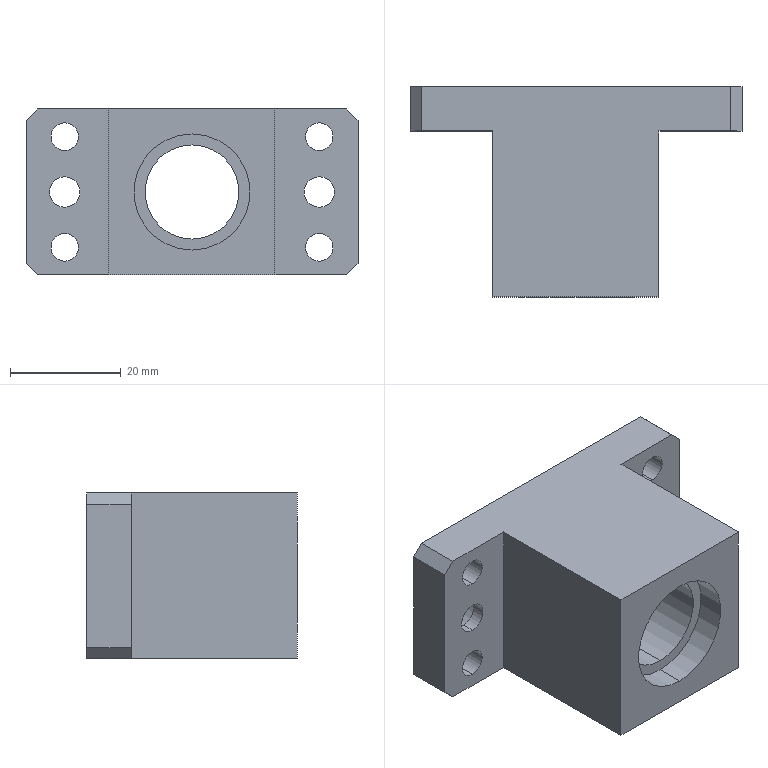Part | NX | features BREP 1 | 1 solid | 40 faces | box 60 x 38 x 30 mm | volume 29884 mm3 | cylinder 22 | plane 18 | commonest cylinder face diameters 5 x8 5.5 x4 10 x4 21 x4 17 x2
STEP:
#1=CARTESIAN_POINT('',(-23.,-8.,-12.5));
#2=VERTEX_POINT('',#1);
#3=CARTESIAN_POINT('',(-23.,-8.,-7.5));
#4=VERTEX_POINT('',#3);
#5=CARTESIAN_POINT('',(-23.,-8.,-10.));
#6=DIRECTION('',(0.,1.,0.));
#7=DIRECTION('',(-1.,0.,0.));
#8=AXIS2_PLACEMENT_3D('',#5,#6,#7);
#9=CIRCLE('',#8,2.5);
#10=EDGE_CURVE('',#2,#4,#9,.T.);
#11=ORIENTED_EDGE('',*,*,#10,.F.);
#12=CARTESIAN_POINT('',(-23.,0.,-12.5));
#13=VERTEX_POINT('',#12);
#14=CARTESIAN_POINT('',(-23.,0.,-12.5));
#15=DIRECTION('',(0.,1.,0.));
#16=VECTOR('',#15,1000.);
#17=LINE('',#14,#16);
#18=EDGE_CURVE('',#2,#13,#17,.T.);
#19=ORIENTED_EDGE('',*,*,#18,.T.);
#20=CARTESIAN_POINT('',(-23.,0.,-7.5));
#21=VERTEX_POINT('',#20);
#22=CARTESIAN_POINT('',(-23.,0.,-10.));
#23=DIRECTION('',(0.,1.,0.));
#24=DIRECTION('',(0.,0.,1.));
#25=AXIS2_PLACEMENT_3D('',#22,#23,#24);
#26=CIRCLE('',#25,2.5);
#27=EDGE_CURVE('',#13,#21,#26,.T.);
#28=ORIENTED_EDGE('',*,*,#27,.T.);
#29=CARTESIAN_POINT('',(-23.,0.,-7.5));
#30=DIRECTION('',(0.,1.,0.));
#31=VECTOR('',#30,1000.);
#32=LINE('',#29,#31);
#33=EDGE_CURVE('',#4,#21,#32,.T.);
#34=ORIENTED_EDGE('',*,*,#33,.F.);
#35=EDGE_LOOP('',(#11,#19,#28,#34));
#36=FACE_BOUND('',#35,.T.);
#37=CARTESIAN_POINT('',(-23.,0.,-10.));
#38=DIRECTION('',(0.,1.,0.));
#39=DIRECTION('',(0.,0.,-1.));
#40=AXIS2_PLACEMENT_3D('',#37,#38,#39);
#41=CYLINDRICAL_SURFACE('',#40,2.5);
#42=ADVANCED_FACE('',(#36),#41,.F.);
#43=CARTESIAN_POINT('',(23.,-8.,-12.5));
#44=VERTEX_POINT('',#43);
#45=CARTESIAN_POINT('',(23.,-8.,-7.5));
#46=VERTEX_POINT('',#45);
#47=CARTESIAN_POINT('',(23.,-8.,-10.));
#48=DIRECTION('',(0.,1.,0.));
#49=DIRECTION('',(-1.,0.,0.));
#50=AXIS2_PLACEMENT_3D('',#47,#48,#49);
#51=CIRCLE('',#50,2.5);
#52=EDGE_CURVE('',#44,#46,#51,.T.);
#53=ORIENTED_EDGE('',*,*,#52,.F.);
#54=CARTESIAN_POINT('',(23.,0.,-12.5));
#55=VERTEX_POINT('',#54);
#56=CARTESIAN_POINT('',(23.,0.,-12.5));
#57=DIRECTION('',(0.,1.,0.));
#58=VECTOR('',#57,1000.);
#59=LINE('',#56,#58);
#60=EDGE_CURVE('',#44,#55,#59,.T.);
#61=ORIENTED_EDGE('',*,*,#60,.T.);
#62=CARTESIAN_POINT('',(23.,0.,-7.5));
#63=VERTEX_POINT('',#62);
#64=CARTESIAN_POINT('',(23.,0.,-10.));
#65=DIRECTION('',(0.,1.,0.));
#66=DIRECTION('',(0.,0.,1.));
#67=AXIS2_PLACEMENT_3D('',#64,#65,#66);
#68=CIRCLE('',#67,2.5);
#69=EDGE_CURVE('',#55,#63,#68,.T.);
#70=ORIENTED_EDGE('',*,*,#69,.T.);
#71=CARTESIAN_POINT('',(23.,0.,-7.5));
#72=DIRECTION('',(0.,1.,0.));
#73=VECTOR('',#72,1000.);
#74=LINE('',#71,#73);
#75=EDGE_CURVE('',#46,#63,#74,.T.);
#76=ORIENTED_EDGE('',*,*,#75,.F.);
#77=EDGE_LOOP('',(#53,#61,#70,#76));
#78=FACE_BOUND('',#77,.T.);
#79=CARTESIAN_POINT('',(23.,0.,-10.));
#80=DIRECTION('',(0.,1.,0.));
#81=DIRECTION('',(0.,0.,-1.));
#82=AXIS2_PLACEMENT_3D('',#79,#80,#81);
#83=CYLINDRICAL_SURFACE('',#82,2.5);
#84=ADVANCED_FACE('',(#78),#83,.F.);
#85=CARTESIAN_POINT('',(23.,-8.,7.5));
#86=VERTEX_POINT('',#85);
#87=CARTESIAN_POINT('',(23.,-8.,12.5));
#88=VERTEX_POINT('',#87);
#89=CARTESIAN_POINT('',(23.,-8.,10.));
#90=DIRECTION('',(0.,1.,0.));
#91=DIRECTION('',(-1.,0.,0.));
#92=AXIS2_PLACEMENT_3D('',#89,#90,#91);
#93=CIRCLE('',#92,2.5);
#94=EDGE_CURVE('',#86,#88,#93,.T.);
#95=ORIENTED_EDGE('',*,*,#94,.F.);
#96=CARTESIAN_POINT('',(23.,0.,7.5));
#97=VERTEX_POINT('',#96);
#98=CARTESIAN_POINT('',(23.,0.,7.5));
#99=DIRECTION('',(0.,1.,0.));
#100=VECTOR('',#99,1000.);
#101=LINE('',#98,#100);
#102=EDGE_CURVE('',#86,#97,#101,.T.);
#103=ORIENTED_EDGE('',*,*,#102,.T.);
#104=CARTESIAN_POINT('',(23.,0.,12.5));
#105=VERTEX_POINT('',#104);
#106=CARTESIAN_POINT('',(23.,0.,10.));
#107=DIRECTION('',(0.,1.,0.));
#108=DIRECTION('',(0.,0.,1.));
#109=AXIS2_PLACEMENT_3D('',#106,#107,#108);
#110=CIRCLE('',#109,2.5);
#111=EDGE_CURVE('',#97,#105,#110,.T.);
#112=ORIENTED_EDGE('',*,*,#111,.T.);
#113=CARTESIAN_POINT('',(23.,0.,12.5));
#114=DIRECTION('',(0.,1.,0.));
#115=VECTOR('',#114,1000.);
#116=LINE('',#113,#115);
#117=EDGE_CURVE('',#88,#105,#116,.T.);
#118=ORIENTED_EDGE('',*,*,#117,.F.);
#119=EDGE_LOOP('',(#95,#103,#112,#118));
#120=FACE_BOUND('',#119,.T.);
#121=CARTESIAN_POINT('',(23.,0.,10.));
#122=DIRECTION('',(0.,1.,0.));
#123=DIRECTION('',(0.,0.,-1.));
#124=AXIS2_PLACEMENT_3D('',#121,#122,#123);
#125=CYLINDRICAL_SURFACE('',#124,2.5);
#126=ADVANCED_FACE('',(#120),#125,.F.);
#127=CARTESIAN_POINT('',(-23.,-8.,7.5));
#128=VERTEX_POINT('',#127);
#129=CARTESIAN_POINT('',(-23.,-8.,12.5));
#130=VERTEX_POINT('',#129);
#131=CARTESIAN_POINT('',(-23.,-8.,10.));
#132=DIRECTION('',(0.,1.,0.));
#133=DIRECTION('',(-1.,0.,0.));
#134=AXIS2_PLACEMENT_3D('',#131,#132,#133);
#135=CIRCLE('',#134,2.5);
#136=EDGE_CURVE('',#128,#130,#135,.T.);
#137=ORIENTED_EDGE('',*,*,#136,.F.);
#138=CARTESIAN_POINT('',(-23.,0.,7.5));
#139=VERTEX_POINT('',#138);
#140=CARTESIAN_POINT('',(-23.,0.,7.5));
#141=DIRECTION('',(0.,1.,0.));
#142=VECTOR('',#141,1000.);
#143=LINE('',#140,#142);
#144=EDGE_CURVE('',#128,#139,#143,.T.);
#145=ORIENTED_EDGE('',*,*,#144,.T.);
#146=CARTESIAN_POINT('',(-23.,0.,12.5));
#147=VERTEX_POINT('',#146);
#148=CARTESIAN_POINT('',(-23.,0.,10.));
#149=DIRECTION('',(0.,1.,0.));
#150=DIRECTION('',(0.,0.,1.));
#151=AXIS2_PLACEMENT_3D('',#148,#149,#150);
#152=CIRCLE('',#151,2.5);
#153=EDGE_CURVE('',#139,#147,#152,.T.);
#154=ORIENTED_EDGE('',*,*,#153,.T.);
#155=CARTESIAN_POINT('',(-23.,0.,12.5));
#156=DIRECTION('',(0.,1.,0.));
#157=VECTOR('',#156,1000.);
#158=LINE('',#155,#157);
#159=EDGE_CURVE('',#130,#147,#158,.T.);
#160=ORIENTED_EDGE('',*,*,#159,.F.);
#161=EDGE_LOOP('',(#137,#145,#154,#160));
#162=FACE_BOUND('',#161,.T.);
#163=CARTESIAN_POINT('',(-23.,0.,10.));
#164=DIRECTION('',(0.,1.,0.));
#165=DIRECTION('',(0.,0.,-1.));
#166=AXIS2_PLACEMENT_3D('',#163,#164,#165);
#167=CYLINDRICAL_SURFACE('',#166,2.5);
#168=ADVANCED_FACE('',(#162),#167,.F.);
#169=CARTESIAN_POINT('',(0.,-33.,8.5));
#170=VERTEX_POINT('',#169);
#171=CARTESIAN_POINT('',(0.,-33.,-8.5));
#172=VERTEX_POINT('',#171);
#173=CARTESIAN_POINT('',(0.,-33.,0.));
#174=DIRECTION('',(0.,-1.,0.));
#175=DIRECTION('',(0.,0.,-1.));
#176=AXIS2_PLACEMENT_3D('',#173,#174,#175);
#177=CIRCLE('',#176,8.5);
#178=EDGE_CURVE('',#170,#172,#177,.T.);
#179=ORIENTED_EDGE('',*,*,#178,.T.);
#180=CARTESIAN_POINT('',(0.,-5.,-8.5));
#181=VERTEX_POINT('',#180);
#182=CARTESIAN_POINT('',(0.,-38.,-8.5));
#183=DIRECTION('',(0.,1.,0.));
#184=VECTOR('',#183,1000.);
#185=LINE('',#182,#184);
#186=EDGE_CURVE('',#172,#181,#185,.T.);
#187=ORIENTED_EDGE('',*,*,#186,.T.);
#188=CARTESIAN_POINT('',(0.,-5.,8.5));
#189=VERTEX_POINT('',#188);
#190=CARTESIAN_POINT('',(0.,-5.,0.));
#191=DIRECTION('',(0.,1.,0.));
#192=DIRECTION('',(0.,0.,1.));
#193=AXIS2_PLACEMENT_3D('',#190,#191,#192);
#194=CIRCLE('',#193,8.5);
#195=EDGE_CURVE('',#181,#189,#194,.T.);
#196=ORIENTED_EDGE('',*,*,#195,.T.);
#197=CARTESIAN_POINT('',(0.,-38.,8.5));
#198=DIRECTION('',(0.,1.,0.));
#199=VECTOR('',#198,1000.);
#200=LINE('',#197,#199);
#201=EDGE_CURVE('',#170,#189,#200,.T.);
#202=ORIENTED_EDGE('',*,*,#201,.F.);
#203=EDGE_LOOP('',(#179,#187,#196,#202));
#204=FACE_BOUND('',#203,.T.);
#205=CARTESIAN_POINT('',(0.,-38.,0.));
#206=DIRECTION('',(0.,1.,0.));
#207=DIRECTION('',(0.,0.,-1.));
#208=AXIS2_PLACEMENT_3D('',#205,#206,#207);
#209=CYLINDRICAL_SURFACE('',#208,8.5);
#210=ADVANCED_FACE('',(#204),#209,.F.);
#211=CARTESIAN_POINT('',(0.,-33.,10.5));
#212=VERTEX_POINT('',#211);
#213=CARTESIAN_POINT('',(0.,-33.,-10.5));
#214=VERTEX_POINT('',#213);
#215=CARTESIAN_POINT('',(0.,-33.,0.));
#216=DIRECTION('',(0.,-1.,0.));
#217=DIRECTION('',(0.,0.,-1.));
#218=AXIS2_PLACEMENT_3D('',#215,#216,#217);
#219=CIRCLE('',#218,10.5);
#220=EDGE_CURVE('',#212,#214,#219,.T.);
#221=ORIENTED_EDGE('',*,*,#220,.F.);
#222=CARTESIAN_POINT('',(0.,-38.,10.5));
#223=VERTEX_POINT('',#222);
#224=CARTESIAN_POINT('',(0.,-33.,10.5));
#225=DIRECTION('',(0.,-1.,0.));
#226=VECTOR('',#225,1000.);
#227=LINE('',#224,#226);
#228=EDGE_CURVE('',#223,#212,#227,.F.);
#229=ORIENTED_EDGE('',*,*,#228,.F.);
#230=CARTESIAN_POINT('',(0.,-38.,-10.5));
#231=VERTEX_POINT('',#230);
#232=CARTESIAN_POINT('',(0.,-38.,0.));
#233=DIRECTION('',(0.,-1.,0.));
#234=DIRECTION('',(0.,0.,-1.));
#235=AXIS2_PLACEMENT_3D('',#232,#233,#234);
#236=CIRCLE('',#235,10.5);
#237=EDGE_CURVE('',#223,#231,#236,.T.);
#238=ORIENTED_EDGE('',*,*,#237,.T.);
#239=CARTESIAN_POINT('',(0.,-33.,-10.5));
#240=DIRECTION('',(0.,-1.,0.));
#241=VECTOR('',#240,1000.);
#242=LINE('',#239,#241);
#243=EDGE_CURVE('',#231,#214,#242,.F.);
#244=ORIENTED_EDGE('',*,*,#243,.T.);
#245=EDGE_LOOP('',(#221,#229,#238,#244));
#246=FACE_BOUND('',#245,.T.);
#247=CARTESIAN_POINT('',(0.,-33.,0.));
#248=DIRECTION('',(0.,-1.,0.));
#249=DIRECTION('',(0.,0.,1.));
#250=AXIS2_PLACEMENT_3D('',#247,#248,#249);
#251=CYLINDRICAL_SURFACE('',#250,10.5);
#252=ADVANCED_FACE('',(#246),#251,.F.);
#253=CARTESIAN_POINT('',(0.,-5.,-10.5));
#254=VERTEX_POINT('',#253);
#255=CARTESIAN_POINT('',(0.,-5.,10.5));
#256=VERTEX_POINT('',#255);
#257=CARTESIAN_POINT('',(0.,-5.,0.));
#258=DIRECTION('',(0.,1.,0.));
#259=DIRECTION('',(0.,0.,1.));
#260=AXIS2_PLACEMENT_3D('',#257,#258,#259);
#261=CIRCLE('',#260,10.5);
#262=EDGE_CURVE('',#254,#256,#261,.T.);
#263=ORIENTED_EDGE('',*,*,#262,.F.);
#264=CARTESIAN_POINT('',(0.,0.,-10.5));
#265=VERTEX_POINT('',#264);
#266=CARTESIAN_POINT('',(0.,-5.,-10.5));
#267=DIRECTION('',(0.,1.,0.));
#268=VECTOR('',#267,1000.);
#269=LINE('',#266,#268);
#270=EDGE_CURVE('',#254,#265,#269,.T.);
#271=ORIENTED_EDGE('',*,*,#270,.T.);
#272=CARTESIAN_POINT('',(0.,0.,10.5));
#273=VERTEX_POINT('',#272);
#274=CARTESIAN_POINT('',(0.,0.,0.));
#275=DIRECTION('',(0.,1.,0.));
#276=DIRECTION('',(0.,0.,1.));
#277=AXIS2_PLACEMENT_3D('',#274,#275,#276);
#278=CIRCLE('',#277,10.5);
#279=EDGE_CURVE('',#265,#273,#278,.T.);
#280=ORIENTED_EDGE('',*,*,#279,.T.);
#281=CARTESIAN_POINT('',(0.,-5.,10.5));
#282=DIRECTION('',(0.,1.,0.));
#283=VECTOR('',#282,1000.);
#284=LINE('',#281,#283);
#285=EDGE_CURVE('',#256,#273,#284,.T.);
#286=ORIENTED_EDGE('',*,*,#285,.F.);
#287=EDGE_LOOP('',(#263,#271,#280,#286));
#288=FACE_BOUND('',#287,.T.);
#289=CARTESIAN_POINT('',(0.,-5.,0.));
#290=DIRECTION('',(0.,1.,0.));
#291=DIRECTION('',(0.,0.,-1.));
#292=AXIS2_PLACEMENT_3D('',#289,#290,#291);
#293=CYLINDRICAL_SURFACE('',#292,10.5);
#294=ADVANCED_FACE('',(#288),#293,.F.);
#295=CARTESIAN_POINT('',(23.,-5.7,-5.));
#296=VERTEX_POINT('',#295);
#297=CARTESIAN_POINT('',(23.,-5.7,5.));
#298=VERTEX_POINT('',#297);
#299=CARTESIAN_POINT('',(23.,-5.7,0.));
#300=DIRECTION('',(0.,1.,0.));
#301=DIRECTION('',(0.,0.,1.));
#302=AXIS2_PLACEMENT_3D('',#299,#300,#301);
#303=CIRCLE('',#302,5.);
#304=EDGE_CURVE('',#296,#298,#303,.T.);
#305=ORIENTED_EDGE('',*,*,#304,.F.);
#306=CARTESIAN_POINT('',(23.,0.,-5.));
#307=VERTEX_POINT('',#306);
#308=CARTESIAN_POINT('',(23.,0.,-5.));
#309=DIRECTION('',(0.,1.,0.));
#310=VECTOR('',#309,1000.);
#311=LINE('',#308,#310);
#312=EDGE_CURVE('',#296,#307,#311,.T.);
#313=ORIENTED_EDGE('',*,*,#312,.T.);
#314=CARTESIAN_POINT('',(23.,0.,5.));
#315=VERTEX_POINT('',#314);
#316=CARTESIAN_POINT('',(23.,0.,0.));
#317=DIRECTION('',(0.,1.,0.));
#318=DIRECTION('',(0.,0.,1.));
#319=AXIS2_PLACEMENT_3D('',#316,#317,#318);
#320=CIRCLE('',#319,5.);
#321=EDGE_CURVE('',#307,#315,#320,.T.);
#322=ORIENTED_EDGE('',*,*,#321,.T.);
#323=CARTESIAN_POINT('',(23.,0.,5.));
#324=DIRECTION('',(0.,1.,0.));
#325=VECTOR('',#324,1000.);
#326=LINE('',#323,#325);
#327=EDGE_CURVE('',#298,#315,#326,.T.);
#328=ORIENTED_EDGE('',*,*,#327,.F.);
#329=EDGE_LOOP('',(#305,#313,#322,#328));
#330=FACE_BOUND('',#329,.T.);
#331=CARTESIAN_POINT('',(23.,0.,0.));
#332=DIRECTION('',(0.,1.,0.));
#333=DIRECTION('',(0.,0.,-1.));
#334=AXIS2_PLACEMENT_3D('',#331,#332,#333);
#335=CYLINDRICAL_SURFACE('',#334,5.);
#336=ADVANCED_FACE('',(#330),#335,.F.);
#337=CARTESIAN_POINT('',(23.,-8.,-2.75));
#338=VERTEX_POINT('',#337);
#339=CARTESIAN_POINT('',(23.,-8.,2.75));
#340=VERTEX_POINT('',#339);
#341=CARTESIAN_POINT('',(23.,-8.,0.));
#342=DIRECTION('',(0.,1.,0.));
#343=DIRECTION('',(-1.,0.,0.));
#344=AXIS2_PLACEMENT_3D('',#341,#342,#343);
#345=CIRCLE('',#344,2.75);
#346=EDGE_CURVE('',#338,#340,#345,.T.);
#347=ORIENTED_EDGE('',*,*,#346,.F.);
#348=CARTESIAN_POINT('',(23.,-5.7,-2.75));
#349=VERTEX_POINT('',#348);
#350=CARTESIAN_POINT('',(23.,0.,-2.75));
#351=DIRECTION('',(0.,1.,0.));
#352=VECTOR('',#351,1000.);
#353=LINE('',#350,#352);
#354=EDGE_CURVE('',#338,#349,#353,.T.);
#355=ORIENTED_EDGE('',*,*,#354,.T.);
#356=CARTESIAN_POINT('',(23.,-5.7,2.75));
#357=VERTEX_POINT('',#356);
#358=CARTESIAN_POINT('',(23.,-5.7,0.));
#359=DIRECTION('',(0.,1.,0.));
#360=DIRECTION('',(0.,0.,1.));
#361=AXIS2_PLACEMENT_3D('',#358,#359,#360);
#362=CIRCLE('',#361,2.75);
#363=EDGE_CURVE('',#349,#357,#362,.T.);
#364=ORIENTED_EDGE('',*,*,#363,.T.);
#365=CARTESIAN_POINT('',(23.,0.,2.75));
#366=DIRECTION('',(0.,1.,0.));
#367=VECTOR('',#366,1000.);
#368=LINE('',#365,#367);
#369=EDGE_CURVE('',#340,#357,#368,.T.);
#370=ORIENTED_EDGE('',*,*,#369,.F.);
#371=EDGE_LOOP('',(#347,#355,#364,#370));
#372=FACE_BOUND('',#371,.T.);
#373=CARTESIAN_POINT('',(23.,0.,0.));
#374=DIRECTION('',(0.,1.,0.));
#375=DIRECTION('',(0.,0.,-1.));
#376=AXIS2_PLACEMENT_3D('',#373,#374,#375);
#377=CYLINDRICAL_SURFACE('',#376,2.75);
#378=ADVANCED_FACE('',(#372),#377,.F.);
#379=CARTESIAN_POINT('',(-23.,-5.7,-5.));
#380=VERTEX_POINT('',#379);
#381=CARTESIAN_POINT('',(-23.,-5.7,5.));
#382=VERTEX_POINT('',#381);
#383=CARTESIAN_POINT('',(-23.,-5.7,0.));
#384=DIRECTION('',(0.,1.,0.));
#385=DIRECTION('',(0.,0.,1.));
#386=AXIS2_PLACEMENT_3D('',#383,#384,#385);
#387=CIRCLE('',#386,5.);
#388=EDGE_CURVE('',#380,#382,#387,.T.);
#389=ORIENTED_EDGE('',*,*,#388,.F.);
#390=CARTESIAN_POINT('',(-23.,0.,-5.));
#391=VERTEX_POINT('',#390);
#392=CARTESIAN_POINT('',(-23.,0.,-5.));
#393=DIRECTION('',(0.,1.,0.));
#394=VECTOR('',#393,1000.);
#395=LINE('',#392,#394);
#396=EDGE_CURVE('',#380,#391,#395,.T.);
#397=ORIENTED_EDGE('',*,*,#396,.T.);
#398=CARTESIAN_POINT('',(-23.,0.,5.));
#399=VERTEX_POINT('',#398);
#400=CARTESIAN_POINT('',(-23.,0.,0.));
#401=DIRECTION('',(0.,1.,0.));
#402=DIRECTION('',(0.,0.,1.));
#403=AXIS2_PLACEMENT_3D('',#400,#401,#402);
#404=CIRCLE('',#403,5.);
#405=EDGE_CURVE('',#391,#399,#404,.T.);
#406=ORIENTED_EDGE('',*,*,#405,.T.);
#407=CARTESIAN_POINT('',(-23.,0.,5.));
#408=DIRECTION('',(0.,1.,0.));
#409=VECTOR('',#408,1000.);
#410=LINE('',#407,#409);
#411=EDGE_CURVE('',#382,#399,#410,.T.);
#412=ORIENTED_EDGE('',*,*,#411,.F.);
#413=EDGE_LOOP('',(#389,#397,#406,#412));
#414=FACE_BOUND('',#413,.T.);
#415=CARTESIAN_POINT('',(-23.,0.,0.));
#416=DIRECTION('',(0.,1.,0.));
#417=DIRECTION('',(0.,0.,-1.));
#418=AXIS2_PLACEMENT_3D('',#415,#416,#417);
#419=CYLINDRICAL_SURFACE('',#418,5.);
#420=ADVANCED_FACE('',(#414),#419,.F.);
#421=CARTESIAN_POINT('',(-23.,-8.,-2.75));
#422=VERTEX_POINT('',#421);
#423=CARTESIAN_POINT('',(-23.,-8.,2.75));
#424=VERTEX_POINT('',#423);
#425=CARTESIAN_POINT('',(-23.,-8.,0.));
#426=DIRECTION('',(0.,1.,0.));
#427=DIRECTION('',(-1.,0.,0.));
#428=AXIS2_PLACEMENT_3D('',#425,#426,#427);
#429=CIRCLE('',#428,2.75);
#430=EDGE_CURVE('',#422,#424,#429,.T.);
#431=ORIENTED_EDGE('',*,*,#430,.F.);
#432=CARTESIAN_POINT('',(-23.,-5.7,-2.75));
#433=VERTEX_POINT('',#432);
#434=CARTESIAN_POINT('',(-23.,0.,-2.75));
#435=DIRECTION('',(0.,1.,0.));
#436=VECTOR('',#435,1000.);
#437=LINE('',#434,#436);
#438=EDGE_CURVE('',#422,#433,#437,.T.);
#439=ORIENTED_EDGE('',*,*,#438,.T.);
#440=CARTESIAN_POINT('',(-23.,-5.7,2.75));
#441=VERTEX_POINT('',#440);
#442=CARTESIAN_POINT('',(-23.,-5.7,0.));
#443=DIRECTION('',(0.,1.,0.));
#444=DIRECTION('',(0.,0.,1.));
#445=AXIS2_PLACEMENT_3D('',#442,#443,#444);
#446=CIRCLE('',#445,2.75);
#447=EDGE_CURVE('',#433,#441,#446,.T.);
#448=ORIENTED_EDGE('',*,*,#447,.T.);
#449=CARTESIAN_POINT('',(-23.,0.,2.75));
#450=DIRECTION('',(0.,1.,0.));
#451=VECTOR('',#450,1000.);
#452=LINE('',#449,#451);
#453=EDGE_CURVE('',#424,#441,#452,.T.);
#454=ORIENTED_EDGE('',*,*,#453,.F.);
#455=EDGE_LOOP('',(#431,#439,#448,#454));
#456=FACE_BOUND('',#455,.T.);
#457=CARTESIAN_POINT('',(-23.,0.,0.));
#458=DIRECTION('',(0.,1.,0.));
#459=DIRECTION('',(0.,0.,-1.));
#460=AXIS2_PLACEMENT_3D('',#457,#458,#459);
#461=CYLINDRICAL_SURFACE('',#460,2.75);
#462=ADVANCED_FACE('',(#456),#461,.F.);
#463=CARTESIAN_POINT('',(30.,-8.,13.));
#464=VERTEX_POINT('',#463);
#465=CARTESIAN_POINT('',(30.,-8.,-13.));
#466=VERTEX_POINT('',#465);
#467=CARTESIAN_POINT('',(30.,-8.,15.));
#468=DIRECTION('',(0.,0.,-1.));
#469=VECTOR('',#468,1000.);
#470=LINE('',#467,#469);
#471=EDGE_CURVE('',#464,#466,#470,.T.);
#472=ORIENTED_EDGE('',*,*,#471,.T.);
#473=CARTESIAN_POINT('',(30.,0.,-13.));
#474=VERTEX_POINT('',#473);
#475=CARTESIAN_POINT('',(30.,0.,-13.));
#476=DIRECTION('',(0.,1.,0.));
#477=VECTOR('',#476,1000.);
#478=LINE('',#475,#477);
#479=EDGE_CURVE('',#466,#474,#478,.T.);
#480=ORIENTED_EDGE('',*,*,#479,.T.);
#481=CARTESIAN_POINT('',(30.,0.,13.));
#482=VERTEX_POINT('',#481);
#483=CARTESIAN_POINT('',(30.,0.,15.));
#484=DIRECTION('',(0.,0.,-1.));
#485=VECTOR('',#484,1000.);
#486=LINE('',#483,#485);
#487=EDGE_CURVE('',#482,#474,#486,.T.);
#488=ORIENTED_EDGE('',*,*,#487,.F.);
#489=CARTESIAN_POINT('',(30.,0.,13.));
#490=DIRECTION('',(0.,-1.,0.));
#491=VECTOR('',#490,1000.);
#492=LINE('',#489,#491);
#493=EDGE_CURVE('',#482,#464,#492,.T.);
#494=ORIENTED_EDGE('',*,*,#493,.T.);
#495=EDGE_LOOP('',(#472,#480,#488,#494));
#496=FACE_BOUND('',#495,.T.);
#497=CARTESIAN_POINT('',(30.,0.,15.));
#498=DIRECTION('',(-1.,0.,0.));
#499=DIRECTION('',(0.,0.,-1.));
#500=AXIS2_PLACEMENT_3D('',#497,#498,#499);
#501=PLANE('',#500);
#502=ADVANCED_FACE('',(#496),#501,.F.);
#503=CARTESIAN_POINT('',(-23.,0.,-10.));
#504=DIRECTION('',(0.,1.,0.));
#505=DIRECTION('',(0.,0.,1.));
#506=AXIS2_PLACEMENT_3D('',#503,#504,#505);
#507=CIRCLE('',#506,2.5);
#508=EDGE_CURVE('',#21,#13,#507,.T.);
#509=ORIENTED_EDGE('',*,*,#508,.F.);
#510=ORIENTED_EDGE('',*,*,#27,.F.);
#511=EDGE_LOOP('',(#509,#510));
#512=FACE_BOUND('',#511,.T.);
#513=CARTESIAN_POINT('',(23.,0.,-10.));
#514=DIRECTION('',(0.,1.,0.));
#515=DIRECTION('',(0.,0.,1.));
#516=AXIS2_PLACEMENT_3D('',#513,#514,#515);
#517=CIRCLE('',#516,2.5);
#518=EDGE_CURVE('',#63,#55,#517,.T.);
#519=ORIENTED_EDGE('',*,*,#518,.F.);
#520=ORIENTED_EDGE('',*,*,#69,.F.);
#521=EDGE_LOOP('',(#519,#520));
#522=FACE_BOUND('',#521,.T.);
#523=CARTESIAN_POINT('',(23.,0.,10.));
#524=DIRECTION('',(0.,1.,0.));
#525=DIRECTION('',(0.,0.,1.));
#526=AXIS2_PLACEMENT_3D('',#523,#524,#525);
#527=CIRCLE('',#526,2.5);
#528=EDGE_CURVE('',#105,#97,#527,.T.);
#529=ORIENTED_EDGE('',*,*,#528,.F.);
#530=ORIENTED_EDGE('',*,*,#111,.F.);
#531=EDGE_LOOP('',(#529,#530));
#532=FACE_BOUND('',#531,.T.);
#533=CARTESIAN_POINT('',(-23.,0.,10.));
#534=DIRECTION('',(0.,1.,0.));
#535=DIRECTION('',(0.,0.,1.));
#536=AXIS2_PLACEMENT_3D('',#533,#534,#535);
#537=CIRCLE('',#536,2.5);
#538=EDGE_CURVE('',#147,#139,#537,.T.);
#539=ORIENTED_EDGE('',*,*,#538,.F.);
#540=ORIENTED_EDGE('',*,*,#153,.F.);
#541=EDGE_LOOP('',(#539,#540));
#542=FACE_BOUND('',#541,.T.);
#543=CARTESIAN_POINT('',(0.,0.,0.));
#544=DIRECTION('',(0.,1.,0.));
#545=DIRECTION('',(0.,0.,1.));
#546=AXIS2_PLACEMENT_3D('',#543,#544,#545);
#547=CIRCLE('',#546,10.5);
#548=EDGE_CURVE('',#273,#265,#547,.T.);
#549=ORIENTED_EDGE('',*,*,#548,.F.);
#550=ORIENTED_EDGE('',*,*,#279,.F.);
#551=EDGE_LOOP('',(#549,#550));
#552=FACE_BOUND('',#551,.T.);
#553=CARTESIAN_POINT('',(23.,0.,0.));
#554=DIRECTION('',(0.,1.,0.));
#555=DIRECTION('',(0.,0.,1.));
#556=AXIS2_PLACEMENT_3D('',#553,#554,#555);
#557=CIRCLE('',#556,5.);
#558=EDGE_CURVE('',#315,#307,#557,.T.);
#559=ORIENTED_EDGE('',*,*,#558,.F.);
#560=ORIENTED_EDGE('',*,*,#321,.F.);
#561=EDGE_LOOP('',(#559,#560));
#562=FACE_BOUND('',#561,.T.);
#563=CARTESIAN_POINT('',(-23.,0.,0.));
#564=DIRECTION('',(0.,1.,0.));
#565=DIRECTION('',(0.,0.,1.));
#566=AXIS2_PLACEMENT_3D('',#563,#564,#565);
#567=CIRCLE('',#566,5.);
#568=EDGE_CURVE('',#399,#391,#567,.T.);
#569=ORIENTED_EDGE('',*,*,#568,.F.);
#570=ORIENTED_EDGE('',*,*,#405,.F.);
#571=EDGE_LOOP('',(#569,#570));
#572=FACE_BOUND('',#571,.T.);
#573=CARTESIAN_POINT('',(28.,0.,-15.));
#574=VERTEX_POINT('',#573);
#575=CARTESIAN_POINT('',(-28.,0.,-15.));
#576=VERTEX_POINT('',#575);
#577=CARTESIAN_POINT('',(-30.,0.,-15.));
#578=DIRECTION('',(-1.,0.,0.));
#579=VECTOR('',#578,1000.);
#580=LINE('',#577,#579);
#581=EDGE_CURVE('',#574,#576,#580,.T.);
#582=ORIENTED_EDGE('',*,*,#581,.T.);
#583=CARTESIAN_POINT('',(-30.,0.,-13.));
#584=VERTEX_POINT('',#583);
#585=CARTESIAN_POINT('',(-30.,0.,-13.));
#586=DIRECTION('',(-0.7071,0.,0.7071));
#587=VECTOR('',#586,1000.);
#588=LINE('',#585,#587);
#589=EDGE_CURVE('',#576,#584,#588,.T.);
#590=ORIENTED_EDGE('',*,*,#589,.T.);
#591=CARTESIAN_POINT('',(-30.,0.,13.));
#592=VERTEX_POINT('',#591);
#593=CARTESIAN_POINT('',(-30.,0.,15.));
#594=DIRECTION('',(0.,0.,-1.));
#595=VECTOR('',#594,1000.);
#596=LINE('',#593,#595);
#597=EDGE_CURVE('',#592,#584,#596,.T.);
#598=ORIENTED_EDGE('',*,*,#597,.F.);
#599=CARTESIAN_POINT('',(-28.,0.,15.));
#600=VERTEX_POINT('',#599);
#601=CARTESIAN_POINT('',(-28.,0.,15.));
#602=DIRECTION('',(0.7071,0.,0.7071));
#603=VECTOR('',#602,1000.);
#604=LINE('',#601,#603);
#605=EDGE_CURVE('',#592,#600,#604,.T.);
#606=ORIENTED_EDGE('',*,*,#605,.T.);
#607=CARTESIAN_POINT('',(28.,0.,15.));
#608=VERTEX_POINT('',#607);
#609=CARTESIAN_POINT('',(-30.,0.,15.));
#610=DIRECTION('',(-1.,0.,0.));
#611=VECTOR('',#610,1000.);
#612=LINE('',#609,#611);
#613=EDGE_CURVE('',#608,#600,#612,.T.);
#614=ORIENTED_EDGE('',*,*,#613,.F.);
#615=CARTESIAN_POINT('',(28.,0.,15.));
#616=DIRECTION('',(0.7071,0.,-0.7071));
#617=VECTOR('',#616,1000.);
#618=LINE('',#615,#617);
#619=EDGE_CURVE('',#608,#482,#618,.T.);
#620=ORIENTED_EDGE('',*,*,#619,.T.);
#621=ORIENTED_EDGE('',*,*,#487,.T.);
#622=CARTESIAN_POINT('',(30.,0.,-13.));
#623=DIRECTION('',(-0.7071,0.,-0.7071));
#624=VECTOR('',#623,1000.);
#625=LINE('',#622,#624);
#626=EDGE_CURVE('',#474,#574,#625,.T.);
#627=ORIENTED_EDGE('',*,*,#626,.T.);
#628=EDGE_LOOP('',(#582,#590,#598,#606,#614,#620,#621,#627));
#629=FACE_BOUND('',#628,.T.);
#630=CARTESIAN_POINT('',(-30.,0.,15.));
#631=DIRECTION('',(0.,-1.,0.));
#632=DIRECTION('',(0.,0.,1.));
#633=AXIS2_PLACEMENT_3D('',#630,#631,#632);
#634=PLANE('',#633);
#635=ADVANCED_FACE('',(#512,#522,#532,#542,#552,#562,#572,#629),#634,.F.);
#636=ORIENTED_EDGE('',*,*,#597,.T.);
#637=CARTESIAN_POINT('',(-30.,-8.,-13.));
#638=VERTEX_POINT('',#637);
#639=CARTESIAN_POINT('',(-30.,-8.,-13.));
#640=DIRECTION('',(0.,-1.,0.));
#641=VECTOR('',#640,1000.);
#642=LINE('',#639,#641);
#643=EDGE_CURVE('',#584,#638,#642,.T.);
#644=ORIENTED_EDGE('',*,*,#643,.T.);
#645=CARTESIAN_POINT('',(-30.,-8.,13.));
#646=VERTEX_POINT('',#645);
#647=CARTESIAN_POINT('',(-30.,-8.,15.));
#648=DIRECTION('',(0.,0.,-1.));
#649=VECTOR('',#648,1000.);
#650=LINE('',#647,#649);
#651=EDGE_CURVE('',#646,#638,#650,.T.);
#652=ORIENTED_EDGE('',*,*,#651,.F.);
#653=CARTESIAN_POINT('',(-30.,0.,13.));
#654=DIRECTION('',(0.,1.,0.));
#655=VECTOR('',#654,1000.);
#656=LINE('',#653,#655);
#657=EDGE_CURVE('',#646,#592,#656,.T.);
#658=ORIENTED_EDGE('',*,*,#657,.T.);
#659=EDGE_LOOP('',(#636,#644,#652,#658));
#660=FACE_BOUND('',#659,.T.);
#661=CARTESIAN_POINT('',(-30.,0.,15.));
#662=DIRECTION('',(1.,0.,0.));
#663=DIRECTION('',(0.,0.,1.));
#664=AXIS2_PLACEMENT_3D('',#661,#662,#663);
#665=PLANE('',#664);
#666=ADVANCED_FACE('',(#660),#665,.F.);
#667=CARTESIAN_POINT('',(-23.,-8.,-10.));
#668=DIRECTION('',(0.,1.,0.));
#669=DIRECTION('',(-1.,0.,0.));
#670=AXIS2_PLACEMENT_3D('',#667,#668,#669);
#671=CIRCLE('',#670,2.5);
#672=EDGE_CURVE('',#4,#2,#671,.T.);
#673=ORIENTED_EDGE('',*,*,#672,.T.);
#674=ORIENTED_EDGE('',*,*,#10,.T.);
#675=EDGE_LOOP('',(#673,#674));
#676=FACE_BOUND('',#675,.T.);
#677=CARTESIAN_POINT('',(-23.,-8.,10.));
#678=DIRECTION('',(0.,1.,0.));
#679=DIRECTION('',(-1.,0.,0.));
#680=AXIS2_PLACEMENT_3D('',#677,#678,#679);
#681=CIRCLE('',#680,2.5);
#682=EDGE_CURVE('',#130,#128,#681,.T.);
#683=ORIENTED_EDGE('',*,*,#682,.T.);
#684=ORIENTED_EDGE('',*,*,#136,.T.);
#685=EDGE_LOOP('',(#683,#684));
#686=FACE_BOUND('',#685,.T.);
#687=CARTESIAN_POINT('',(-23.,-8.,0.));
#688=DIRECTION('',(0.,1.,0.));
#689=DIRECTION('',(-1.,0.,0.));
#690=AXIS2_PLACEMENT_3D('',#687,#688,#689);
#691=CIRCLE('',#690,2.75);
#692=EDGE_CURVE('',#424,#422,#691,.T.);
#693=ORIENTED_EDGE('',*,*,#692,.T.);
#694=ORIENTED_EDGE('',*,*,#430,.T.);
#695=EDGE_LOOP('',(#693,#694));
#696=FACE_BOUND('',#695,.T.);
#697=ORIENTED_EDGE('',*,*,#651,.T.);
#698=CARTESIAN_POINT('',(-28.,-8.,-15.));
#699=VERTEX_POINT('',#698);
#700=CARTESIAN_POINT('',(-30.,-8.,-13.));
#701=DIRECTION('',(0.7071,0.,-0.7071));
#702=VECTOR('',#701,1000.);
#703=LINE('',#700,#702);
#704=EDGE_CURVE('',#638,#699,#703,.T.);
#705=ORIENTED_EDGE('',*,*,#704,.T.);
#706=CARTESIAN_POINT('',(-15.,-8.,-15.));
#707=VERTEX_POINT('',#706);
#708=CARTESIAN_POINT('',(-30.,-8.,-15.));
#709=DIRECTION('',(1.,0.,0.));
#710=VECTOR('',#709,1000.);
#711=LINE('',#708,#710);
#712=EDGE_CURVE('',#699,#707,#711,.T.);
#713=ORIENTED_EDGE('',*,*,#712,.T.);
#714=CARTESIAN_POINT('',(-15.,-8.,15.));
#715=VERTEX_POINT('',#714);
#716=CARTESIAN_POINT('',(-15.,-8.,15.));
#717=DIRECTION('',(0.,0.,-1.));
#718=VECTOR('',#717,1000.);
#719=LINE('',#716,#718);
#720=EDGE_CURVE('',#715,#707,#719,.T.);
#721=ORIENTED_EDGE('',*,*,#720,.F.);
#722=CARTESIAN_POINT('',(-28.,-8.,15.));
#723=VERTEX_POINT('',#722);
#724=CARTESIAN_POINT('',(-30.,-8.,15.));
#725=DIRECTION('',(1.,0.,0.));
#726=VECTOR('',#725,1000.);
#727=LINE('',#724,#726);
#728=EDGE_CURVE('',#723,#715,#727,.T.);
#729=ORIENTED_EDGE('',*,*,#728,.F.);
#730=CARTESIAN_POINT('',(-28.,-8.,15.));
#731=DIRECTION('',(-0.7071,0.,-0.7071));
#732=VECTOR('',#731,1000.);
#733=LINE('',#730,#732);
#734=EDGE_CURVE('',#723,#646,#733,.T.);
#735=ORIENTED_EDGE('',*,*,#734,.T.);
#736=EDGE_LOOP('',(#697,#705,#713,#721,#729,#735));
#737=FACE_BOUND('',#736,.T.);
#738=CARTESIAN_POINT('',(-30.,-8.,15.));
#739=DIRECTION('',(0.,1.,0.));
#740=DIRECTION('',(1.,0.,0.));
#741=AXIS2_PLACEMENT_3D('',#738,#739,#740);
#742=PLANE('',#741);
#743=ADVANCED_FACE('',(#676,#686,#696,#737),#742,.F.);
#744=CARTESIAN_POINT('',(-15.,-38.,-15.));
#745=VERTEX_POINT('',#744);
#746=CARTESIAN_POINT('',(-15.,-8.,-15.));
#747=DIRECTION('',(0.,-1.,0.));
#748=VECTOR('',#747,1000.);
#749=LINE('',#746,#748);
#750=EDGE_CURVE('',#707,#745,#749,.T.);
#751=ORIENTED_EDGE('',*,*,#750,.T.);
#752=CARTESIAN_POINT('',(-15.,-38.,15.));
#753=VERTEX_POINT('',#752);
#754=CARTESIAN_POINT('',(-15.,-38.,15.));
#755=DIRECTION('',(0.,0.,-1.));
#756=VECTOR('',#755,1000.);
#757=LINE('',#754,#756);
#758=EDGE_CURVE('',#753,#745,#757,.T.);
#759=ORIENTED_EDGE('',*,*,#758,.F.);
#760=CARTESIAN_POINT('',(-15.,-8.,15.));
#761=DIRECTION('',(0.,-1.,0.));
#762=VECTOR('',#761,1000.);
#763=LINE('',#760,#762);
#764=EDGE_CURVE('',#715,#753,#763,.T.);
#765=ORIENTED_EDGE('',*,*,#764,.F.);
#766=ORIENTED_EDGE('',*,*,#720,.T.);
#767=EDGE_LOOP('',(#751,#759,#765,#766));
#768=FACE_BOUND('',#767,.T.);
#769=CARTESIAN_POINT('',(-15.,-8.,15.));
#770=DIRECTION('',(1.,0.,0.));
#771=DIRECTION('',(0.,-1.,0.));
#772=AXIS2_PLACEMENT_3D('',#769,#770,#771);
#773=PLANE('',#772);
#774=ADVANCED_FACE('',(#768),#773,.F.);
#775=CARTESIAN_POINT('',(0.,-38.,0.));
#776=DIRECTION('',(0.,-1.,0.));
#777=DIRECTION('',(0.,0.,-1.));
#778=AXIS2_PLACEMENT_3D('',#775,#776,#777);
#779=CIRCLE('',#778,10.5);
#780=EDGE_CURVE('',#231,#223,#779,.T.);
#781=ORIENTED_EDGE('',*,*,#780,.F.);
#782=ORIENTED_EDGE('',*,*,#237,.F.);
#783=EDGE_LOOP('',(#781,#782));
#784=FACE_BOUND('',#783,.T.);
#785=CARTESIAN_POINT('',(15.,-38.,-15.));
#786=VERTEX_POINT('',#785);
#787=CARTESIAN_POINT('',(15.,-38.,-15.));
#788=DIRECTION('',(1.,0.,0.));
#789=VECTOR('',#788,1000.);
#790=LINE('',#787,#789);
#791=EDGE_CURVE('',#745,#786,#790,.T.);
#792=ORIENTED_EDGE('',*,*,#791,.T.);
#793=CARTESIAN_POINT('',(15.,-38.,15.));
#794=VERTEX_POINT('',#793);
#795=CARTESIAN_POINT('',(15.,-38.,15.));
#796=DIRECTION('',(0.,0.,-1.));
#797=VECTOR('',#796,1000.);
#798=LINE('',#795,#797);
#799=EDGE_CURVE('',#794,#786,#798,.T.);
#800=ORIENTED_EDGE('',*,*,#799,.F.);
#801=CARTESIAN_POINT('',(15.,-38.,15.));
#802=DIRECTION('',(1.,0.,0.));
#803=VECTOR('',#802,1000.);
#804=LINE('',#801,#803);
#805=EDGE_CURVE('',#753,#794,#804,.T.);
#806=ORIENTED_EDGE('',*,*,#805,.F.);
#807=ORIENTED_EDGE('',*,*,#758,.T.);
#808=EDGE_LOOP('',(#792,#800,#806,#807));
#809=FACE_BOUND('',#808,.T.);
#810=CARTESIAN_POINT('',(15.,-38.,15.));
#811=DIRECTION('',(0.,1.,0.));
#812=DIRECTION('',(0.,0.,-1.));
#813=AXIS2_PLACEMENT_3D('',#810,#811,#812);
#814=PLANE('',#813);
#815=ADVANCED_FACE('',(#784,#809),#814,.F.);
#816=CARTESIAN_POINT('',(15.,-8.,-15.));
#817=VERTEX_POINT('',#816);
#818=CARTESIAN_POINT('',(15.,-8.,-15.));
#819=DIRECTION('',(0.,1.,0.));
#820=VECTOR('',#819,1000.);
#821=LINE('',#818,#820);
#822=EDGE_CURVE('',#786,#817,#821,.T.);
#823=ORIENTED_EDGE('',*,*,#822,.T.);
#824=CARTESIAN_POINT('',(15.,-8.,15.));
#825=VERTEX_POINT('',#824);
#826=CARTESIAN_POINT('',(15.,-8.,15.));
#827=DIRECTION('',(0.,0.,-1.));
#828=VECTOR('',#827,1000.);
#829=LINE('',#826,#828);
#830=EDGE_CURVE('',#825,#817,#829,.T.);
#831=ORIENTED_EDGE('',*,*,#830,.F.);
#832=CARTESIAN_POINT('',(15.,-8.,15.));
#833=DIRECTION('',(0.,1.,0.));
#834=VECTOR('',#833,1000.);
#835=LINE('',#832,#834);
#836=EDGE_CURVE('',#794,#825,#835,.T.);
#837=ORIENTED_EDGE('',*,*,#836,.F.);
#838=ORIENTED_EDGE('',*,*,#799,.T.);
#839=EDGE_LOOP('',(#823,#831,#837,#838));
#840=FACE_BOUND('',#839,.T.);
#841=CARTESIAN_POINT('',(15.,-8.,15.));
#842=DIRECTION('',(-1.,0.,0.));
#843=DIRECTION('',(0.,1.,0.));
#844=AXIS2_PLACEMENT_3D('',#841,#842,#843);
#845=PLANE('',#844);
#846=ADVANCED_FACE('',(#840),#845,.F.);
#847=CARTESIAN_POINT('',(23.,-8.,-10.));
#848=DIRECTION('',(0.,1.,0.));
#849=DIRECTION('',(-1.,0.,0.));
#850=AXIS2_PLACEMENT_3D('',#847,#848,#849);
#851=CIRCLE('',#850,2.5);
#852=EDGE_CURVE('',#46,#44,#851,.T.);
#853=ORIENTED_EDGE('',*,*,#852,.T.);
#854=ORIENTED_EDGE('',*,*,#52,.T.);
#855=EDGE_LOOP('',(#853,#854));
#856=FACE_BOUND('',#855,.T.);
#857=CARTESIAN_POINT('',(23.,-8.,10.));
#858=DIRECTION('',(0.,1.,0.));
#859=DIRECTION('',(-1.,0.,0.));
#860=AXIS2_PLACEMENT_3D('',#857,#858,#859);
#861=CIRCLE('',#860,2.5);
#862=EDGE_CURVE('',#88,#86,#861,.T.);
#863=ORIENTED_EDGE('',*,*,#862,.T.);
#864=ORIENTED_EDGE('',*,*,#94,.T.);
#865=EDGE_LOOP('',(#863,#864));
#866=FACE_BOUND('',#865,.T.);
#867=CARTESIAN_POINT('',(23.,-8.,0.));
#868=DIRECTION('',(0.,1.,0.));
#869=DIRECTION('',(-1.,0.,0.));
#870=AXIS2_PLACEMENT_3D('',#867,#868,#869);
#871=CIRCLE('',#870,2.75);
#872=EDGE_CURVE('',#340,#338,#871,.T.);
#873=ORIENTED_EDGE('',*,*,#872,.T.);
#874=ORIENTED_EDGE('',*,*,#346,.T.);
#875=EDGE_LOOP('',(#873,#874));
#876=FACE_BOUND('',#875,.T.);
#877=CARTESIAN_POINT('',(28.,-8.,-15.));
#878=VERTEX_POINT('',#877);
#879=CARTESIAN_POINT('',(30.,-8.,-15.));
#880=DIRECTION('',(1.,0.,0.));
#881=VECTOR('',#880,1000.);
#882=LINE('',#879,#881);
#883=EDGE_CURVE('',#817,#878,#882,.T.);
#884=ORIENTED_EDGE('',*,*,#883,.T.);
#885=CARTESIAN_POINT('',(30.,-8.,-13.));
#886=DIRECTION('',(0.7071,0.,0.7071));
#887=VECTOR('',#886,1000.);
#888=LINE('',#885,#887);
#889=EDGE_CURVE('',#878,#466,#888,.T.);
#890=ORIENTED_EDGE('',*,*,#889,.T.);
#891=ORIENTED_EDGE('',*,*,#471,.F.);
#892=CARTESIAN_POINT('',(28.,-8.,15.));
#893=VERTEX_POINT('',#892);
#894=CARTESIAN_POINT('',(28.,-8.,15.));
#895=DIRECTION('',(-0.7071,0.,0.7071));
#896=VECTOR('',#895,1000.);
#897=LINE('',#894,#896);
#898=EDGE_CURVE('',#464,#893,#897,.T.);
#899=ORIENTED_EDGE('',*,*,#898,.T.);
#900=CARTESIAN_POINT('',(30.,-8.,15.));
#901=DIRECTION('',(1.,0.,0.));
#902=VECTOR('',#901,1000.);
#903=LINE('',#900,#902);
#904=EDGE_CURVE('',#825,#893,#903,.T.);
#905=ORIENTED_EDGE('',*,*,#904,.F.);
#906=ORIENTED_EDGE('',*,*,#830,.T.);
#907=EDGE_LOOP('',(#884,#890,#891,#899,#905,#906));
#908=FACE_BOUND('',#907,.T.);
#909=CARTESIAN_POINT('',(30.,-8.,15.));
#910=DIRECTION('',(0.,1.,0.));
#911=DIRECTION('',(1.,0.,0.));
#912=AXIS2_PLACEMENT_3D('',#909,#910,#911);
#913=PLANE('',#912);
#914=ADVANCED_FACE('',(#856,#866,#876,#908),#913,.F.);
#915=ORIENTED_EDGE('',*,*,#613,.T.);
#916=CARTESIAN_POINT('',(-28.,0.,15.));
#917=DIRECTION('',(0.,-1.,0.));
#918=VECTOR('',#917,1000.);
#919=LINE('',#916,#918);
#920=EDGE_CURVE('',#600,#723,#919,.T.);
#921=ORIENTED_EDGE('',*,*,#920,.T.);
#922=ORIENTED_EDGE('',*,*,#728,.T.);
#923=ORIENTED_EDGE('',*,*,#764,.T.);
#924=ORIENTED_EDGE('',*,*,#805,.T.);
#925=ORIENTED_EDGE('',*,*,#836,.T.);
#926=ORIENTED_EDGE('',*,*,#904,.T.);
#927=CARTESIAN_POINT('',(28.,0.,15.));
#928=DIRECTION('',(0.,1.,0.));
#929=VECTOR('',#928,1000.);
#930=LINE('',#927,#929);
#931=EDGE_CURVE('',#893,#608,#930,.T.);
#932=ORIENTED_EDGE('',*,*,#931,.T.);
#933=EDGE_LOOP('',(#915,#921,#922,#923,#924,#925,#926,#932));
#934=FACE_BOUND('',#933,.T.);
#935=CARTESIAN_POINT('',(0.,0.,15.));
#936=DIRECTION('',(0.,0.,-1.));
#937=DIRECTION('',(1.,0.,0.));
#938=AXIS2_PLACEMENT_3D('',#935,#936,#937);
#939=PLANE('',#938);
#940=ADVANCED_FACE('',(#934),#939,.F.);
#941=ORIENTED_EDGE('',*,*,#712,.F.);
#942=CARTESIAN_POINT('',(-28.,0.,-15.));
#943=DIRECTION('',(0.,1.,0.));
#944=VECTOR('',#943,1000.);
#945=LINE('',#942,#944);
#946=EDGE_CURVE('',#699,#576,#945,.T.);
#947=ORIENTED_EDGE('',*,*,#946,.T.);
#948=ORIENTED_EDGE('',*,*,#581,.F.);
#949=CARTESIAN_POINT('',(28.,-8.,-15.));
#950=DIRECTION('',(0.,-1.,0.));
#951=VECTOR('',#950,1000.);
#952=LINE('',#949,#951);
#953=EDGE_CURVE('',#574,#878,#952,.T.);
#954=ORIENTED_EDGE('',*,*,#953,.T.);
#955=ORIENTED_EDGE('',*,*,#883,.F.);
#956=ORIENTED_EDGE('',*,*,#822,.F.);
#957=ORIENTED_EDGE('',*,*,#791,.F.);
#958=ORIENTED_EDGE('',*,*,#750,.F.);
#959=EDGE_LOOP('',(#941,#947,#948,#954,#955,#956,#957,#958));
#960=FACE_BOUND('',#959,.T.);
#961=CARTESIAN_POINT('',(0.,0.,-15.));
#962=DIRECTION('',(0.,0.,-1.));
#963=DIRECTION('',(1.,0.,0.));
#964=AXIS2_PLACEMENT_3D('',#961,#962,#963);
#965=PLANE('',#964);
#966=ADVANCED_FACE('',(#960),#965,.T.);
#967=ORIENTED_EDGE('',*,*,#438,.F.);
#968=ORIENTED_EDGE('',*,*,#692,.F.);
#969=ORIENTED_EDGE('',*,*,#453,.T.);
#970=CARTESIAN_POINT('',(-23.,-5.7,0.));
#971=DIRECTION('',(0.,1.,0.));
#972=DIRECTION('',(0.,0.,1.));
#973=AXIS2_PLACEMENT_3D('',#970,#971,#972);
#974=CIRCLE('',#973,2.75);
#975=EDGE_CURVE('',#441,#433,#974,.T.);
#976=ORIENTED_EDGE('',*,*,#975,.T.);
#977=EDGE_LOOP('',(#967,#968,#969,#976));
#978=FACE_BOUND('',#977,.T.);
#979=CARTESIAN_POINT('',(-23.,0.,0.));
#980=DIRECTION('',(0.,1.,0.));
#981=DIRECTION('',(0.,0.,-1.));
#982=AXIS2_PLACEMENT_3D('',#979,#980,#981);
#983=CYLINDRICAL_SURFACE('',#982,2.75);
#984=ADVANCED_FACE('',(#978),#983,.F.);
#985=ORIENTED_EDGE('',*,*,#975,.F.);
#986=ORIENTED_EDGE('',*,*,#447,.F.);
#987=EDGE_LOOP('',(#985,#986));
#988=FACE_BOUND('',#987,.T.);
#989=CARTESIAN_POINT('',(-23.,-5.7,0.));
#990=DIRECTION('',(0.,1.,0.));
#991=DIRECTION('',(0.,0.,1.));
#992=AXIS2_PLACEMENT_3D('',#989,#990,#991);
#993=CIRCLE('',#992,5.);
#994=EDGE_CURVE('',#382,#380,#993,.T.);
#995=ORIENTED_EDGE('',*,*,#994,.T.);
#996=ORIENTED_EDGE('',*,*,#388,.T.);
#997=EDGE_LOOP('',(#995,#996));
#998=FACE_BOUND('',#997,.T.);
#999=CARTESIAN_POINT('',(-20.25,-5.7,0.));
#1000=DIRECTION('',(0.,-1.,0.));
#1001=DIRECTION('',(0.,0.,1.));
#1002=AXIS2_PLACEMENT_3D('',#999,#1000,#1001);
#1003=PLANE('',#1002);
#1004=ADVANCED_FACE('',(#988,#998),#1003,.F.);
#1005=ORIENTED_EDGE('',*,*,#396,.F.);
#1006=ORIENTED_EDGE('',*,*,#994,.F.);
#1007=ORIENTED_EDGE('',*,*,#411,.T.);
#1008=ORIENTED_EDGE('',*,*,#568,.T.);
#1009=EDGE_LOOP('',(#1005,#1006,#1007,#1008));
#1010=FACE_BOUND('',#1009,.T.);
#1011=CARTESIAN_POINT('',(-23.,0.,0.));
#1012=DIRECTION('',(0.,1.,0.));
#1013=DIRECTION('',(0.,0.,-1.));
#1014=AXIS2_PLACEMENT_3D('',#1011,#1012,#1013);
#1015=CYLINDRICAL_SURFACE('',#1014,5.);
#1016=ADVANCED_FACE('',(#1010),#1015,.F.);
#1017=ORIENTED_EDGE('',*,*,#354,.F.);
#1018=ORIENTED_EDGE('',*,*,#872,.F.);
#1019=ORIENTED_EDGE('',*,*,#369,.T.);
#1020=CARTESIAN_POINT('',(23.,-5.7,0.));
#1021=DIRECTION('',(0.,1.,0.));
#1022=DIRECTION('',(0.,0.,1.));
#1023=AXIS2_PLACEMENT_3D('',#1020,#1021,#1022);
#1024=CIRCLE('',#1023,2.75);
#1025=EDGE_CURVE('',#357,#349,#1024,.T.);
#1026=ORIENTED_EDGE('',*,*,#1025,.T.);
#1027=EDGE_LOOP('',(#1017,#1018,#1019,#1026));
#1028=FACE_BOUND('',#1027,.T.);
#1029=CARTESIAN_POINT('',(23.,0.,0.));
#1030=DIRECTION('',(0.,1.,0.));
#1031=DIRECTION('',(0.,0.,-1.));
#1032=AXIS2_PLACEMENT_3D('',#1029,#1030,#1031);
#1033=CYLINDRICAL_SURFACE('',#1032,2.75);
#1034=ADVANCED_FACE('',(#1028),#1033,.F.);
#1035=ORIENTED_EDGE('',*,*,#1025,.F.);
#1036=ORIENTED_EDGE('',*,*,#363,.F.);
#1037=EDGE_LOOP('',(#1035,#1036));
#1038=FACE_BOUND('',#1037,.T.);
#1039=CARTESIAN_POINT('',(23.,-5.7,0.));
#1040=DIRECTION('',(0.,1.,0.));
#1041=DIRECTION('',(0.,0.,1.));
#1042=AXIS2_PLACEMENT_3D('',#1039,#1040,#1041);
#1043=CIRCLE('',#1042,5.);
#1044=EDGE_CURVE('',#298,#296,#1043,.T.);
#1045=ORIENTED_EDGE('',*,*,#1044,.T.);
#1046=ORIENTED_EDGE('',*,*,#304,.T.);
#1047=EDGE_LOOP('',(#1045,#1046));
#1048=FACE_BOUND('',#1047,.T.);
#1049=CARTESIAN_POINT('',(25.75,-5.7,0.));
#1050=DIRECTION('',(0.,-1.,0.));
#1051=DIRECTION('',(0.,0.,1.));
#1052=AXIS2_PLACEMENT_3D('',#1049,#1050,#1051);
#1053=PLANE('',#1052);
#1054=ADVANCED_FACE('',(#1038,#1048),#1053,.F.);
#1055=ORIENTED_EDGE('',*,*,#312,.F.);
#1056=ORIENTED_EDGE('',*,*,#1044,.F.);
#1057=ORIENTED_EDGE('',*,*,#327,.T.);
#1058=ORIENTED_EDGE('',*,*,#558,.T.);
#1059=EDGE_LOOP('',(#1055,#1056,#1057,#1058));
#1060=FACE_BOUND('',#1059,.T.);
#1061=CARTESIAN_POINT('',(23.,0.,0.));
#1062=DIRECTION('',(0.,1.,0.));
#1063=DIRECTION('',(0.,0.,-1.));
#1064=AXIS2_PLACEMENT_3D('',#1061,#1062,#1063);
#1065=CYLINDRICAL_SURFACE('',#1064,5.);
#1066=ADVANCED_FACE('',(#1060),#1065,.F.);
#1067=ORIENTED_EDGE('',*,*,#589,.F.);
#1068=ORIENTED_EDGE('',*,*,#946,.F.);
#1069=ORIENTED_EDGE('',*,*,#704,.F.);
#1070=ORIENTED_EDGE('',*,*,#643,.F.);
#1071=EDGE_LOOP('',(#1067,#1068,#1069,#1070));
#1072=FACE_BOUND('',#1071,.T.);
#1073=CARTESIAN_POINT('',(-30.,0.,-13.));
#1074=DIRECTION('',(-0.7071,0.,-0.7071));
#1075=DIRECTION('',(0.,-1.,0.));
#1076=AXIS2_PLACEMENT_3D('',#1073,#1074,#1075);
#1077=PLANE('',#1076);
#1078=ADVANCED_FACE('',(#1072),#1077,.T.);
#1079=ORIENTED_EDGE('',*,*,#605,.F.);
#1080=ORIENTED_EDGE('',*,*,#657,.F.);
#1081=ORIENTED_EDGE('',*,*,#734,.F.);
#1082=ORIENTED_EDGE('',*,*,#920,.F.);
#1083=EDGE_LOOP('',(#1079,#1080,#1081,#1082));
#1084=FACE_BOUND('',#1083,.T.);
#1085=CARTESIAN_POINT('',(-28.,0.,15.));
#1086=DIRECTION('',(0.7071,0.,-0.7071));
#1087=DIRECTION('',(0.,1.,0.));
#1088=AXIS2_PLACEMENT_3D('',#1085,#1086,#1087);
#1089=PLANE('',#1088);
#1090=ADVANCED_FACE('',(#1084),#1089,.F.);
#1091=ORIENTED_EDGE('',*,*,#889,.F.);
#1092=ORIENTED_EDGE('',*,*,#953,.F.);
#1093=ORIENTED_EDGE('',*,*,#626,.F.);
#1094=ORIENTED_EDGE('',*,*,#479,.F.);
#1095=EDGE_LOOP('',(#1091,#1092,#1093,#1094));
#1096=FACE_BOUND('',#1095,.T.);
#1097=CARTESIAN_POINT('',(30.,0.,-13.));
#1098=DIRECTION('',(0.7071,0.,-0.7071));
#1099=DIRECTION('',(0.,1.,0.));
#1100=AXIS2_PLACEMENT_3D('',#1097,#1098,#1099);
#1101=PLANE('',#1100);
#1102=ADVANCED_FACE('',(#1096),#1101,.T.);
#1103=ORIENTED_EDGE('',*,*,#898,.F.);
#1104=ORIENTED_EDGE('',*,*,#493,.F.);
#1105=ORIENTED_EDGE('',*,*,#619,.F.);
#1106=ORIENTED_EDGE('',*,*,#931,.F.);
#1107=EDGE_LOOP('',(#1103,#1104,#1105,#1106));
#1108=FACE_BOUND('',#1107,.T.);
#1109=CARTESIAN_POINT('',(28.,0.,15.));
#1110=DIRECTION('',(-0.7071,0.,-0.7071));
#1111=DIRECTION('',(0.,-1.,0.));
#1112=AXIS2_PLACEMENT_3D('',#1109,#1110,#1111);
#1113=PLANE('',#1112);
#1114=ADVANCED_FACE('',(#1108),#1113,.F.);
#1115=ORIENTED_EDGE('',*,*,#270,.F.);
#1116=CARTESIAN_POINT('',(0.,-5.,0.));
#1117=DIRECTION('',(0.,1.,0.));
#1118=DIRECTION('',(0.,0.,1.));
#1119=AXIS2_PLACEMENT_3D('',#1116,#1117,#1118);
#1120=CIRCLE('',#1119,10.5);
#1121=EDGE_CURVE('',#256,#254,#1120,.T.);
#1122=ORIENTED_EDGE('',*,*,#1121,.F.);
#1123=ORIENTED_EDGE('',*,*,#285,.T.);
#1124=ORIENTED_EDGE('',*,*,#548,.T.);
#1125=EDGE_LOOP('',(#1115,#1122,#1123,#1124));
#1126=FACE_BOUND('',#1125,.T.);
#1127=CARTESIAN_POINT('',(0.,-5.,0.));
#1128=DIRECTION('',(0.,1.,0.));
#1129=DIRECTION('',(0.,0.,-1.));
#1130=AXIS2_PLACEMENT_3D('',#1127,#1128,#1129);
#1131=CYLINDRICAL_SURFACE('',#1130,10.5);
#1132=ADVANCED_FACE('',(#1126),#1131,.F.);
#1133=CARTESIAN_POINT('',(0.,-5.,0.));
#1134=DIRECTION('',(0.,1.,0.));
#1135=DIRECTION('',(0.,0.,1.));
#1136=AXIS2_PLACEMENT_3D('',#1133,#1134,#1135);
#1137=CIRCLE('',#1136,8.5);
#1138=EDGE_CURVE('',#189,#181,#1137,.T.);
#1139=ORIENTED_EDGE('',*,*,#1138,.F.);
#1140=ORIENTED_EDGE('',*,*,#195,.F.);
#1141=EDGE_LOOP('',(#1139,#1140));
#1142=FACE_BOUND('',#1141,.T.);
#1143=ORIENTED_EDGE('',*,*,#1121,.T.);
#1144=ORIENTED_EDGE('',*,*,#262,.T.);
#1145=EDGE_LOOP('',(#1143,#1144));
#1146=FACE_BOUND('',#1145,.T.);
#1147=CARTESIAN_POINT('',(0.,-5.,0.));
#1148=DIRECTION('',(0.,1.,0.));
#1149=DIRECTION('',(0.,0.,-1.));
#1150=AXIS2_PLACEMENT_3D('',#1147,#1148,#1149);
#1151=PLANE('',#1150);
#1152=ADVANCED_FACE('',(#1142,#1146),#1151,.T.);
#1153=ORIENTED_EDGE('',*,*,#228,.T.);
#1154=CARTESIAN_POINT('',(0.,-33.,0.));
#1155=DIRECTION('',(0.,-1.,0.));
#1156=DIRECTION('',(0.,0.,-1.));
#1157=AXIS2_PLACEMENT_3D('',#1154,#1155,#1156);
#1158=CIRCLE('',#1157,10.5);
#1159=EDGE_CURVE('',#214,#212,#1158,.T.);
#1160=ORIENTED_EDGE('',*,*,#1159,.F.);
#1161=ORIENTED_EDGE('',*,*,#243,.F.);
#1162=ORIENTED_EDGE('',*,*,#780,.T.);
#1163=EDGE_LOOP('',(#1153,#1160,#1161,#1162));
#1164=FACE_BOUND('',#1163,.T.);
#1165=CARTESIAN_POINT('',(0.,-33.,0.));
#1166=DIRECTION('',(0.,-1.,0.));
#1167=DIRECTION('',(0.,0.,1.));
#1168=AXIS2_PLACEMENT_3D('',#1165,#1166,#1167);
#1169=CYLINDRICAL_SURFACE('',#1168,10.5);
#1170=ADVANCED_FACE('',(#1164),#1169,.F.);
#1171=ORIENTED_EDGE('',*,*,#178,.F.);
#1172=CARTESIAN_POINT('',(0.,-33.,0.));
#1173=DIRECTION('',(0.,-1.,0.));
#1174=DIRECTION('',(0.,0.,-1.));
#1175=AXIS2_PLACEMENT_3D('',#1172,#1173,#1174);
#1176=CIRCLE('',#1175,8.5);
#1177=EDGE_CURVE('',#172,#170,#1176,.T.);
#1178=ORIENTED_EDGE('',*,*,#1177,.F.);
#1179=EDGE_LOOP('',(#1171,#1178));
#1180=FACE_BOUND('',#1179,.T.);
#1181=ORIENTED_EDGE('',*,*,#1159,.T.);
#1182=ORIENTED_EDGE('',*,*,#220,.T.);
#1183=EDGE_LOOP('',(#1181,#1182));
#1184=FACE_BOUND('',#1183,.T.);
#1185=CARTESIAN_POINT('',(0.,-33.,0.));
#1186=DIRECTION('',(0.,-1.,0.));
#1187=DIRECTION('',(0.,0.,1.));
#1188=AXIS2_PLACEMENT_3D('',#1185,#1186,#1187);
#1189=PLANE('',#1188);
#1190=ADVANCED_FACE('',(#1180,#1184),#1189,.T.);
#1191=ORIENTED_EDGE('',*,*,#186,.F.);
#1192=ORIENTED_EDGE('',*,*,#1177,.T.);
#1193=ORIENTED_EDGE('',*,*,#201,.T.);
#1194=ORIENTED_EDGE('',*,*,#1138,.T.);
#1195=EDGE_LOOP('',(#1191,#1192,#1193,#1194));
#1196=FACE_BOUND('',#1195,.T.);
#1197=CARTESIAN_POINT('',(0.,-38.,0.));
#1198=DIRECTION('',(0.,1.,0.));
#1199=DIRECTION('',(0.,0.,-1.));
#1200=AXIS2_PLACEMENT_3D('',#1197,#1198,#1199);
#1201=CYLINDRICAL_SURFACE('',#1200,8.5);
#1202=ADVANCED_FACE('',(#1196),#1201,.F.);
#1203=ORIENTED_EDGE('',*,*,#144,.F.);
#1204=ORIENTED_EDGE('',*,*,#682,.F.);
#1205=ORIENTED_EDGE('',*,*,#159,.T.);
#1206=ORIENTED_EDGE('',*,*,#538,.T.);
#1207=EDGE_LOOP('',(#1203,#1204,#1205,#1206));
#1208=FACE_BOUND('',#1207,.T.);
#1209=CARTESIAN_POINT('',(-23.,0.,10.));
#1210=DIRECTION('',(0.,1.,0.));
#1211=DIRECTION('',(0.,0.,-1.));
#1212=AXIS2_PLACEMENT_3D('',#1209,#1210,#1211);
#1213=CYLINDRICAL_SURFACE('',#1212,2.5);
#1214=ADVANCED_FACE('',(#1208),#1213,.F.);
#1215=ORIENTED_EDGE('',*,*,#102,.F.);
#1216=ORIENTED_EDGE('',*,*,#862,.F.);
#1217=ORIENTED_EDGE('',*,*,#117,.T.);
#1218=ORIENTED_EDGE('',*,*,#528,.T.);
#1219=EDGE_LOOP('',(#1215,#1216,#1217,#1218));
#1220=FACE_BOUND('',#1219,.T.);
#1221=CARTESIAN_POINT('',(23.,0.,10.));
#1222=DIRECTION('',(0.,1.,0.));
#1223=DIRECTION('',(0.,0.,-1.));
#1224=AXIS2_PLACEMENT_3D('',#1221,#1222,#1223);
#1225=CYLINDRICAL_SURFACE('',#1224,2.5);
#1226=ADVANCED_FACE('',(#1220),#1225,.F.);
#1227=ORIENTED_EDGE('',*,*,#60,.F.);
#1228=ORIENTED_EDGE('',*,*,#852,.F.);
#1229=ORIENTED_EDGE('',*,*,#75,.T.);
#1230=ORIENTED_EDGE('',*,*,#518,.T.);
#1231=EDGE_LOOP('',(#1227,#1228,#1229,#1230));
#1232=FACE_BOUND('',#1231,.T.);
#1233=CARTESIAN_POINT('',(23.,0.,-10.));
#1234=DIRECTION('',(0.,1.,0.));
#1235=DIRECTION('',(0.,0.,-1.));
#1236=AXIS2_PLACEMENT_3D('',#1233,#1234,#1235);
#1237=CYLINDRICAL_SURFACE('',#1236,2.5);
#1238=ADVANCED_FACE('',(#1232),#1237,.F.);
#1239=ORIENTED_EDGE('',*,*,#18,.F.);
#1240=ORIENTED_EDGE('',*,*,#672,.F.);
#1241=ORIENTED_EDGE('',*,*,#33,.T.);
#1242=ORIENTED_EDGE('',*,*,#508,.T.);
#1243=EDGE_LOOP('',(#1239,#1240,#1241,#1242));
#1244=FACE_BOUND('',#1243,.T.);
#1245=CARTESIAN_POINT('',(-23.,0.,-10.));
#1246=DIRECTION('',(0.,1.,0.));
#1247=DIRECTION('',(0.,0.,-1.));
#1248=AXIS2_PLACEMENT_3D('',#1245,#1246,#1247);
#1249=CYLINDRICAL_SURFACE('',#1248,2.5);
#1250=ADVANCED_FACE('',(#1244),#1249,.F.);
#1251=CLOSED_SHELL('',(#42,#84,#126,#168,#210,#252,#294,#336,#378,#420,#462,#502,#635,#666,#743,#774,#815,#846,#914,#940,#966,#984,#1004,#1016,#1034,#1054,#1066,#1078,#1090,#1102,#1114,#1132,#1152,#1170,#1190,#1202,#1214,#1226,#1238,#1250));
#1252=MANIFOLD_SOLID_BREP('',#1251);
#1253=(LENGTH_UNIT()NAMED_UNIT(*)SI_UNIT(.MILLI.,.METRE.));
#1254=UNCERTAINTY_MEASURE_WITH_UNIT(LENGTH_MEASURE(0.00001),#1253,'','');
#1255=(NAMED_UNIT(*)PLANE_ANGLE_UNIT()SI_UNIT($,.RADIAN.));
#1256=(NAMED_UNIT(*)SI_UNIT($,.STERADIAN.)SOLID_ANGLE_UNIT());
#1257=(GEOMETRIC_REPRESENTATION_CONTEXT(3)GLOBAL_UNCERTAINTY_ASSIGNED_CONTEXT((#1254))GLOBAL_UNIT_ASSIGNED_CONTEXT((#1253,#1255,#1256))REPRESENTATION_CONTEXT('',''));
#1258=ADVANCED_BREP_SHAPE_REPRESENTATION('',(#1252),#1257);